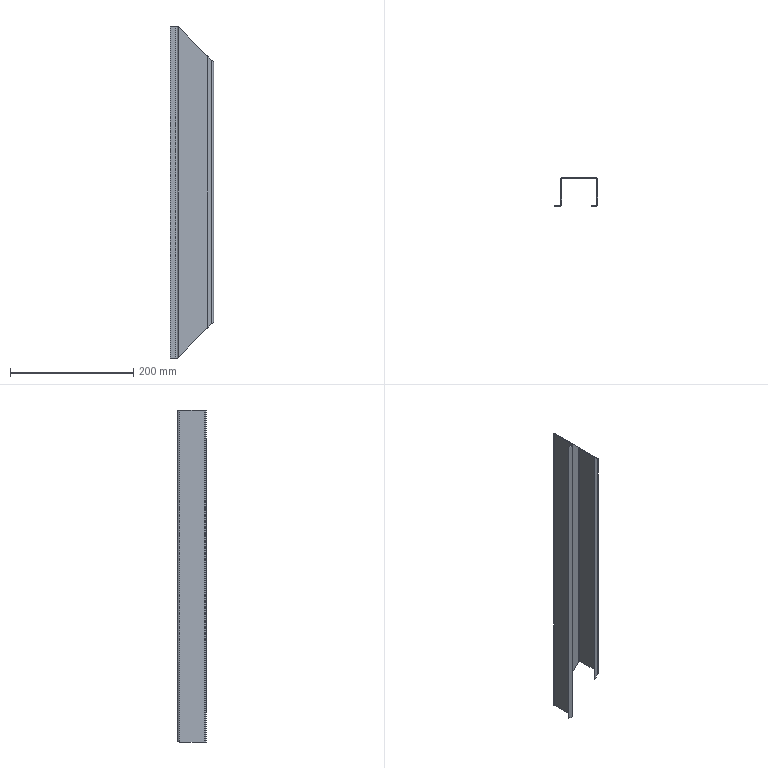Part | STEP file | 750078415 | 1 solid | 34 faces | box 70 x 46.5 x 539 mm | volume 119069 mm3 | plane 20 | cylinder 8 | spline 6 | commonest cylinder face diameters 3 x4 6 x4
STEP:
#1=CARTESIAN_POINT('',(-68.5,43.5,268.));
#2=VERTEX_POINT('',#1);
#3=CARTESIAN_POINT('',(-68.5,43.5,-268.));
#4=VERTEX_POINT('',#3);
#5=CARTESIAN_POINT('',(-68.5,43.5,269.5));
#6=DIRECTION('',(0.,0.,-1.));
#7=VECTOR('',#6,1000.);
#8=LINE('',#5,#7);
#9=EDGE_CURVE('',#2,#4,#8,.T.);
#10=ORIENTED_EDGE('',*,*,#9,.T.);
#11=CARTESIAN_POINT('',(-14.5,43.5,-214.));
#12=VERTEX_POINT('',#11);
#13=CARTESIAN_POINT('',(-68.5,43.5,-268.));
#14=DIRECTION('',(0.7071,0.,0.7071));
#15=VECTOR('',#14,1000.);
#16=LINE('',#13,#15);
#17=EDGE_CURVE('',#4,#12,#16,.T.);
#18=ORIENTED_EDGE('',*,*,#17,.T.);
#19=CARTESIAN_POINT('',(-14.5,43.5,214.));
#20=VERTEX_POINT('',#19);
#21=CARTESIAN_POINT('',(-14.5,43.5,269.5));
#22=DIRECTION('',(0.,0.,1.));
#23=VECTOR('',#22,1000.);
#24=LINE('',#21,#23);
#25=EDGE_CURVE('',#12,#20,#24,.T.);
#26=ORIENTED_EDGE('',*,*,#25,.T.);
#27=CARTESIAN_POINT('',(-14.5,43.5,214.));
#28=DIRECTION('',(-0.7071,0.,0.7071));
#29=VECTOR('',#28,1000.);
#30=LINE('',#27,#29);
#31=EDGE_CURVE('',#20,#2,#30,.T.);
#32=ORIENTED_EDGE('',*,*,#31,.T.);
#33=EDGE_LOOP('',(#10,#18,#26,#32));
#34=FACE_OUTER_BOUND('',#33,.T.);
#35=CARTESIAN_POINT('',(-11.5,43.5,269.5));
#36=DIRECTION('',(0.,-1.,0.));
#37=DIRECTION('',(1.,0.,0.));
#38=AXIS2_PLACEMENT_3D('',#35,#36,#37);
#39=PLANE('',#38);
#40=ADVANCED_FACE('',(#34),#39,.T.);
#41=CARTESIAN_POINT('',(-14.5,45.,-214.));
#42=VERTEX_POINT('',#41);
#43=CARTESIAN_POINT('',(-14.5,44.25,-214.));
#44=DIRECTION('',(0.,-1.,0.));
#45=VECTOR('',#44,1000.);
#46=LINE('',#43,#45);
#47=EDGE_CURVE('',#42,#12,#46,.T.);
#48=ORIENTED_EDGE('',*,*,#47,.T.);
#49=ORIENTED_EDGE('',*,*,#17,.F.);
#50=CARTESIAN_POINT('',(-68.5,45.,-268.));
#51=VERTEX_POINT('',#50);
#52=CARTESIAN_POINT('',(-68.5,44.25,-268.));
#53=DIRECTION('',(0.,1.,0.));
#54=VECTOR('',#53,1000.);
#55=LINE('',#52,#54);
#56=EDGE_CURVE('',#4,#51,#55,.T.);
#57=ORIENTED_EDGE('',*,*,#56,.T.);
#58=CARTESIAN_POINT('',(228.75,45.,29.25));
#59=DIRECTION('',(0.7071,0.,0.7071));
#60=VECTOR('',#59,1000.);
#61=LINE('',#58,#60);
#62=EDGE_CURVE('',#51,#42,#61,.T.);
#63=ORIENTED_EDGE('',*,*,#62,.T.);
#64=EDGE_LOOP('',(#48,#49,#57,#63));
#65=FACE_OUTER_BOUND('',#64,.T.);
#66=CARTESIAN_POINT('',(228.75,45.,29.25));
#67=DIRECTION('',(0.7071,0.,-0.7071));
#68=DIRECTION('',(-0.7071,0.,-0.7071));
#69=AXIS2_PLACEMENT_3D('',#66,#67,#68);
#70=PLANE('',#69);
#71=ADVANCED_FACE('',(#65),#70,.T.);
#72=CARTESIAN_POINT('',(-70.,42.,269.5));
#73=VERTEX_POINT('',#72);
#74=CARTESIAN_POINT('',(-70.,42.,269.5));
#75=CARTESIAN_POINT('',(-70.,42.75,269.5));
#76=CARTESIAN_POINT('',(-69.5,43.5,269.));
#77=CARTESIAN_POINT('',(-68.5,43.5,268.));
#78=(BOUNDED_CURVE()B_SPLINE_CURVE(3,(#74,#75,#76,#77),.UNSPECIFIED.,.F.,.F.)B_SPLINE_CURVE_WITH_KNOTS((4,4),(0.,0.002854),.UNSPECIFIED.)CURVE()GEOMETRIC_REPRESENTATION_ITEM()RATIONAL_B_SPLINE_CURVE((1.,0.6667,0.5,0.5))REPRESENTATION_ITEM(''));
#79=EDGE_CURVE('',#73,#2,#78,.T.);
#80=ORIENTED_EDGE('',*,*,#79,.F.);
#81=CARTESIAN_POINT('',(-70.,42.,-269.5));
#82=VERTEX_POINT('',#81);
#83=CARTESIAN_POINT('',(-70.,42.,269.5));
#84=DIRECTION('',(0.,0.,1.));
#85=VECTOR('',#84,1000.);
#86=LINE('',#83,#85);
#87=EDGE_CURVE('',#82,#73,#86,.T.);
#88=ORIENTED_EDGE('',*,*,#87,.F.);
#89=CARTESIAN_POINT('',(-68.5,43.5,-268.));
#90=CARTESIAN_POINT('',(-69.5,43.5,-269.));
#91=CARTESIAN_POINT('',(-70.,42.75,-269.5));
#92=CARTESIAN_POINT('',(-70.,42.,-269.5));
#93=(BOUNDED_CURVE()B_SPLINE_CURVE(3,(#89,#90,#91,#92),.UNSPECIFIED.,.F.,.F.)B_SPLINE_CURVE_WITH_KNOTS((4,4),(0.,0.002839),.UNSPECIFIED.)CURVE()GEOMETRIC_REPRESENTATION_ITEM()RATIONAL_B_SPLINE_CURVE((0.5,0.5,0.6667,1.))REPRESENTATION_ITEM(''));
#94=EDGE_CURVE('',#4,#82,#93,.T.);
#95=ORIENTED_EDGE('',*,*,#94,.F.);
#96=ORIENTED_EDGE('',*,*,#9,.F.);
#97=EDGE_LOOP('',(#80,#88,#95,#96));
#98=FACE_OUTER_BOUND('',#97,.T.);
#99=CARTESIAN_POINT('',(-68.5,42.,269.5));
#100=DIRECTION('',(0.,0.,-1.));
#101=DIRECTION('',(-1.,0.,0.));
#102=AXIS2_PLACEMENT_3D('',#99,#100,#101);
#103=CYLINDRICAL_SURFACE('',#102,1.5);
#104=ADVANCED_FACE('',(#98),#103,.F.);
#105=CARTESIAN_POINT('',(-68.5,45.,268.));
#106=VERTEX_POINT('',#105);
#107=CARTESIAN_POINT('',(-68.5,45.,268.));
#108=DIRECTION('',(0.,-1.,0.));
#109=VECTOR('',#108,1000.);
#110=LINE('',#107,#109);
#111=EDGE_CURVE('',#106,#2,#110,.T.);
#112=ORIENTED_EDGE('',*,*,#111,.T.);
#113=ORIENTED_EDGE('',*,*,#31,.F.);
#114=CARTESIAN_POINT('',(-14.5,45.,214.));
#115=VERTEX_POINT('',#114);
#116=CARTESIAN_POINT('',(-14.5,44.25,214.));
#117=DIRECTION('',(0.,1.,0.));
#118=VECTOR('',#117,1000.);
#119=LINE('',#116,#118);
#120=EDGE_CURVE('',#20,#115,#119,.T.);
#121=ORIENTED_EDGE('',*,*,#120,.T.);
#122=CARTESIAN_POINT('',(-40.75,45.,240.25));
#123=DIRECTION('',(-0.7071,0.,0.7071));
#124=VECTOR('',#123,1000.);
#125=LINE('',#122,#124);
#126=EDGE_CURVE('',#115,#106,#125,.T.);
#127=ORIENTED_EDGE('',*,*,#126,.T.);
#128=EDGE_LOOP('',(#112,#113,#121,#127));
#129=FACE_OUTER_BOUND('',#128,.T.);
#130=CARTESIAN_POINT('',(-40.75,45.,240.25));
#131=DIRECTION('',(0.7071,0.,0.7071));
#132=DIRECTION('',(0.7071,0.,-0.7071));
#133=AXIS2_PLACEMENT_3D('',#130,#131,#132);
#134=PLANE('',#133);
#135=ADVANCED_FACE('',(#129),#134,.T.);
#136=CARTESIAN_POINT('',(-13.,42.,211.));
#137=VERTEX_POINT('',#136);
#138=CARTESIAN_POINT('',(-14.5,43.5,214.));
#139=CARTESIAN_POINT('',(-13.5,43.5,212.));
#140=CARTESIAN_POINT('',(-13.,42.75,211.));
#141=CARTESIAN_POINT('',(-13.,42.,211.));
#142=(BOUNDED_CURVE()B_SPLINE_CURVE(3,(#138,#139,#140,#141),.UNSPECIFIED.,.F.,.F.)B_SPLINE_CURVE_WITH_KNOTS((4,4),(0.,0.003921),.UNSPECIFIED.)CURVE()GEOMETRIC_REPRESENTATION_ITEM()RATIONAL_B_SPLINE_CURVE((0.5,0.5,0.6667,1.))REPRESENTATION_ITEM(''));
#143=EDGE_CURVE('',#20,#137,#142,.T.);
#144=ORIENTED_EDGE('',*,*,#143,.F.);
#145=ORIENTED_EDGE('',*,*,#25,.F.);
#146=CARTESIAN_POINT('',(-13.,42.,-211.));
#147=VERTEX_POINT('',#146);
#148=CARTESIAN_POINT('',(-13.,42.,-211.));
#149=CARTESIAN_POINT('',(-13.,42.75,-211.));
#150=CARTESIAN_POINT('',(-13.5,43.5,-212.));
#151=CARTESIAN_POINT('',(-14.5,43.5,-214.));
#152=(BOUNDED_CURVE()B_SPLINE_CURVE(3,(#148,#149,#150,#151),.UNSPECIFIED.,.F.,.F.)B_SPLINE_CURVE_WITH_KNOTS((4,4),(0.,0.003968),.UNSPECIFIED.)CURVE()GEOMETRIC_REPRESENTATION_ITEM()RATIONAL_B_SPLINE_CURVE((1.,0.6667,0.5,0.5))REPRESENTATION_ITEM(''));
#153=EDGE_CURVE('',#147,#12,#152,.T.);
#154=ORIENTED_EDGE('',*,*,#153,.F.);
#155=CARTESIAN_POINT('',(-13.,42.,269.5));
#156=DIRECTION('',(0.,0.,-1.));
#157=VECTOR('',#156,1000.);
#158=LINE('',#155,#157);
#159=EDGE_CURVE('',#137,#147,#158,.T.);
#160=ORIENTED_EDGE('',*,*,#159,.F.);
#161=EDGE_LOOP('',(#144,#145,#154,#160));
#162=FACE_OUTER_BOUND('',#161,.T.);
#163=CARTESIAN_POINT('',(-14.5,42.,269.5));
#164=DIRECTION('',(0.,0.,-1.));
#165=DIRECTION('',(-1.,0.,0.));
#166=AXIS2_PLACEMENT_3D('',#163,#164,#165);
#167=CYLINDRICAL_SURFACE('',#166,1.5);
#168=ADVANCED_FACE('',(#162),#167,.F.);
#169=CARTESIAN_POINT('',(-14.5,45.,269.5));
#170=DIRECTION('',(0.,0.,1.));
#171=VECTOR('',#170,1000.);
#172=LINE('',#169,#171);
#173=EDGE_CURVE('',#42,#115,#172,.T.);
#174=ORIENTED_EDGE('',*,*,#173,.F.);
#175=ORIENTED_EDGE('',*,*,#62,.F.);
#176=CARTESIAN_POINT('',(-68.5,45.,269.5));
#177=DIRECTION('',(0.,0.,-1.));
#178=VECTOR('',#177,1000.);
#179=LINE('',#176,#178);
#180=EDGE_CURVE('',#106,#51,#179,.T.);
#181=ORIENTED_EDGE('',*,*,#180,.F.);
#182=ORIENTED_EDGE('',*,*,#126,.F.);
#183=EDGE_LOOP('',(#174,#175,#181,#182));
#184=FACE_OUTER_BOUND('',#183,.T.);
#185=CARTESIAN_POINT('',(-11.5,45.,269.5));
#186=DIRECTION('',(0.,-1.,0.));
#187=DIRECTION('',(1.,0.,0.));
#188=AXIS2_PLACEMENT_3D('',#185,#186,#187);
#189=PLANE('',#188);
#190=ADVANCED_FACE('',(#184),#189,.F.);
#191=ORIENTED_EDGE('',*,*,#79,.T.);
#192=ORIENTED_EDGE('',*,*,#111,.F.);
#193=CARTESIAN_POINT('',(-71.5,42.,269.5));
#194=VERTEX_POINT('',#193);
#195=CARTESIAN_POINT('',(-71.5,42.,269.5));
#196=CARTESIAN_POINT('',(-71.5,43.5,269.5));
#197=CARTESIAN_POINT('',(-70.5,45.,269.));
#198=CARTESIAN_POINT('',(-68.5,45.,268.));
#199=(BOUNDED_CURVE()B_SPLINE_CURVE(3,(#195,#196,#197,#198),.UNSPECIFIED.,.F.,.F.)B_SPLINE_CURVE_WITH_KNOTS((4,4),(0.,0.00499),.UNSPECIFIED.)CURVE()GEOMETRIC_REPRESENTATION_ITEM()RATIONAL_B_SPLINE_CURVE((1.,0.6667,0.5,0.5))REPRESENTATION_ITEM(''));
#200=EDGE_CURVE('',#194,#106,#199,.T.);
#201=ORIENTED_EDGE('',*,*,#200,.F.);
#202=CARTESIAN_POINT('',(-71.5,42.,269.5));
#203=DIRECTION('',(-1.,0.,0.));
#204=VECTOR('',#203,1000.);
#205=LINE('',#202,#204);
#206=EDGE_CURVE('',#73,#194,#205,.T.);
#207=ORIENTED_EDGE('',*,*,#206,.F.);
#208=EDGE_LOOP('',(#191,#192,#201,#207));
#209=FACE_OUTER_BOUND('',#208,.T.);
#210=CARTESIAN_POINT('',(-67.,42.,266.5));
#211=CARTESIAN_POINT('',(-66.5,42.,266.5));
#212=CARTESIAN_POINT('',(-66.,42.,266.5));
#213=CARTESIAN_POINT('',(-65.5,42.,266.5));
#214=CARTESIAN_POINT('',(-67.,45.,266.5));
#215=CARTESIAN_POINT('',(-66.5,46.,266.5));
#216=CARTESIAN_POINT('',(-66.,47.,266.5));
#217=CARTESIAN_POINT('',(-65.5,48.,266.5));
#218=CARTESIAN_POINT('',(-70.,45.,269.5));
#219=CARTESIAN_POINT('',(-70.5,46.,269.5));
#220=CARTESIAN_POINT('',(-71.,47.,269.5));
#221=CARTESIAN_POINT('',(-71.5,48.,269.5));
#222=CARTESIAN_POINT('',(-70.,42.,269.5));
#223=CARTESIAN_POINT('',(-70.5,42.,269.5));
#224=CARTESIAN_POINT('',(-71.,42.,269.5));
#225=CARTESIAN_POINT('',(-71.5,42.,269.5));
#226=CARTESIAN_POINT('',(-70.,39.,269.5));
#227=CARTESIAN_POINT('',(-70.5,38.,269.5));
#228=CARTESIAN_POINT('',(-71.,37.,269.5));
#229=CARTESIAN_POINT('',(-71.5,36.,269.5));
#230=CARTESIAN_POINT('',(-67.,39.,266.5));
#231=CARTESIAN_POINT('',(-66.5,38.,266.5));
#232=CARTESIAN_POINT('',(-66.,37.,266.5));
#233=CARTESIAN_POINT('',(-65.5,36.,266.5));
#234=CARTESIAN_POINT('',(-67.,42.,266.5));
#235=CARTESIAN_POINT('',(-66.5,42.,266.5));
#236=CARTESIAN_POINT('',(-66.,42.,266.5));
#237=CARTESIAN_POINT('',(-65.5,42.,266.5));
#238=(BOUNDED_SURFACE()B_SPLINE_SURFACE(3,3,((#210,#211,#212,#213),(#214,#215,#216,#217),(#218,#219,#220,#221),(#222,#223,#224,#225),(#226,#227,#228,#229),(#230,#231,#232,#233),(#234,#235,#236,#237)),.UNSPECIFIED.,.T.,.F.,.F.)B_SPLINE_SURFACE_WITH_KNOTS((4,3,4),(4,4),(0.,0.5,1.),(0.,1.),.UNSPECIFIED.)GEOMETRIC_REPRESENTATION_ITEM()RATIONAL_B_SPLINE_SURFACE(((1.,1.,1.,1.),(0.3333,0.3333,0.3333,0.3333),(0.3333,0.3333,0.3333,0.3333),(1.,1.,1.,1.),(0.3333,0.3333,0.3333,0.3333),(0.3333,0.3333,0.3333,0.3333),(1.,1.,1.,1.)))REPRESENTATION_ITEM('')SURFACE());
#239=ADVANCED_FACE('',(#209),#238,.F.);
#240=CARTESIAN_POINT('',(-70.,1.5,269.5));
#241=VERTEX_POINT('',#240);
#242=CARTESIAN_POINT('',(-70.,45.,269.5));
#243=DIRECTION('',(0.,-1.,0.));
#244=VECTOR('',#243,1000.);
#245=LINE('',#242,#244);
#246=EDGE_CURVE('',#73,#241,#245,.T.);
#247=ORIENTED_EDGE('',*,*,#246,.T.);
#248=CARTESIAN_POINT('',(-70.,1.5,-269.5));
#249=VERTEX_POINT('',#248);
#250=CARTESIAN_POINT('',(-70.,1.5,269.5));
#251=DIRECTION('',(0.,0.,-1.));
#252=VECTOR('',#251,1000.);
#253=LINE('',#250,#252);
#254=EDGE_CURVE('',#241,#249,#253,.T.);
#255=ORIENTED_EDGE('',*,*,#254,.T.);
#256=CARTESIAN_POINT('',(-70.,45.,-269.5));
#257=DIRECTION('',(0.,1.,0.));
#258=VECTOR('',#257,1000.);
#259=LINE('',#256,#258);
#260=EDGE_CURVE('',#249,#82,#259,.T.);
#261=ORIENTED_EDGE('',*,*,#260,.T.);
#262=ORIENTED_EDGE('',*,*,#87,.T.);
#263=EDGE_LOOP('',(#247,#255,#261,#262));
#264=FACE_OUTER_BOUND('',#263,.T.);
#265=CARTESIAN_POINT('',(-70.,45.,269.5));
#266=DIRECTION('',(1.,0.,0.));
#267=DIRECTION('',(0.,0.,-1.));
#268=AXIS2_PLACEMENT_3D('',#265,#266,#267);
#269=PLANE('',#268);
#270=ADVANCED_FACE('',(#264),#269,.T.);
#271=ORIENTED_EDGE('',*,*,#94,.T.);
#272=CARTESIAN_POINT('',(-71.5,42.,-269.5));
#273=VERTEX_POINT('',#272);
#274=CARTESIAN_POINT('',(-70.75,42.,-269.5));
#275=DIRECTION('',(1.,0.,0.));
#276=VECTOR('',#275,1000.);
#277=LINE('',#274,#276);
#278=EDGE_CURVE('',#273,#82,#277,.T.);
#279=ORIENTED_EDGE('',*,*,#278,.F.);
#280=CARTESIAN_POINT('',(-68.5,45.,-268.));
#281=CARTESIAN_POINT('',(-70.5,45.,-269.));
#282=CARTESIAN_POINT('',(-71.5,43.5,-269.5));
#283=CARTESIAN_POINT('',(-71.5,42.,-269.5));
#284=(BOUNDED_CURVE()B_SPLINE_CURVE(3,(#280,#281,#282,#283),.UNSPECIFIED.,.F.,.F.)B_SPLINE_CURVE_WITH_KNOTS((4,4),(0.,0.004967),.UNSPECIFIED.)CURVE()GEOMETRIC_REPRESENTATION_ITEM()RATIONAL_B_SPLINE_CURVE((0.5,0.5,0.6667,1.))REPRESENTATION_ITEM(''));
#285=EDGE_CURVE('',#51,#273,#284,.T.);
#286=ORIENTED_EDGE('',*,*,#285,.F.);
#287=ORIENTED_EDGE('',*,*,#56,.F.);
#288=EDGE_LOOP('',(#271,#279,#286,#287));
#289=FACE_OUTER_BOUND('',#288,.T.);
#290=CARTESIAN_POINT('',(-70.,42.,-269.5));
#291=CARTESIAN_POINT('',(-70.5,42.,-269.5));
#292=CARTESIAN_POINT('',(-71.,42.,-269.5));
#293=CARTESIAN_POINT('',(-71.5,42.,-269.5));
#294=CARTESIAN_POINT('',(-70.,45.,-269.5));
#295=CARTESIAN_POINT('',(-70.5,46.,-269.5));
#296=CARTESIAN_POINT('',(-71.,47.,-269.5));
#297=CARTESIAN_POINT('',(-71.5,48.,-269.5));
#298=CARTESIAN_POINT('',(-67.,45.,-266.5));
#299=CARTESIAN_POINT('',(-66.5,46.,-266.5));
#300=CARTESIAN_POINT('',(-66.,47.,-266.5));
#301=CARTESIAN_POINT('',(-65.5,48.,-266.5));
#302=CARTESIAN_POINT('',(-67.,42.,-266.5));
#303=CARTESIAN_POINT('',(-66.5,42.,-266.5));
#304=CARTESIAN_POINT('',(-66.,42.,-266.5));
#305=CARTESIAN_POINT('',(-65.5,42.,-266.5));
#306=CARTESIAN_POINT('',(-67.,39.,-266.5));
#307=CARTESIAN_POINT('',(-66.5,38.,-266.5));
#308=CARTESIAN_POINT('',(-66.,37.,-266.5));
#309=CARTESIAN_POINT('',(-65.5,36.,-266.5));
#310=CARTESIAN_POINT('',(-70.,39.,-269.5));
#311=CARTESIAN_POINT('',(-70.5,38.,-269.5));
#312=CARTESIAN_POINT('',(-71.,37.,-269.5));
#313=CARTESIAN_POINT('',(-71.5,36.,-269.5));
#314=CARTESIAN_POINT('',(-70.,42.,-269.5));
#315=CARTESIAN_POINT('',(-70.5,42.,-269.5));
#316=CARTESIAN_POINT('',(-71.,42.,-269.5));
#317=CARTESIAN_POINT('',(-71.5,42.,-269.5));
#318=(BOUNDED_SURFACE()B_SPLINE_SURFACE(3,3,((#290,#291,#292,#293),(#294,#295,#296,#297),(#298,#299,#300,#301),(#302,#303,#304,#305),(#306,#307,#308,#309),(#310,#311,#312,#313),(#314,#315,#316,#317)),.UNSPECIFIED.,.T.,.F.,.F.)B_SPLINE_SURFACE_WITH_KNOTS((4,3,4),(4,4),(0.,0.5,1.),(0.,1.),.UNSPECIFIED.)GEOMETRIC_REPRESENTATION_ITEM()RATIONAL_B_SPLINE_SURFACE(((1.,1.,1.,1.),(0.3333,0.3333,0.3333,0.3333),(0.3333,0.3333,0.3333,0.3333),(1.,1.,1.,1.),(0.3333,0.3333,0.3333,0.3333),(0.3333,0.3333,0.3333,0.3333),(1.,1.,1.,1.)))REPRESENTATION_ITEM('')SURFACE());
#319=ADVANCED_FACE('',(#289),#318,.F.);
#320=ORIENTED_EDGE('',*,*,#159,.T.);
#321=CARTESIAN_POINT('',(-13.,1.5,-211.));
#322=VERTEX_POINT('',#321);
#323=CARTESIAN_POINT('',(-13.,-1.5,-211.));
#324=DIRECTION('',(0.,-1.,0.));
#325=VECTOR('',#324,1000.);
#326=LINE('',#323,#325);
#327=EDGE_CURVE('',#147,#322,#326,.T.);
#328=ORIENTED_EDGE('',*,*,#327,.T.);
#329=CARTESIAN_POINT('',(-13.,1.5,211.));
#330=VERTEX_POINT('',#329);
#331=CARTESIAN_POINT('',(-13.,1.5,269.5));
#332=DIRECTION('',(0.,0.,1.));
#333=VECTOR('',#332,1000.);
#334=LINE('',#331,#333);
#335=EDGE_CURVE('',#322,#330,#334,.T.);
#336=ORIENTED_EDGE('',*,*,#335,.T.);
#337=CARTESIAN_POINT('',(-13.,-1.5,211.));
#338=DIRECTION('',(0.,1.,0.));
#339=VECTOR('',#338,1000.);
#340=LINE('',#337,#339);
#341=EDGE_CURVE('',#330,#137,#340,.T.);
#342=ORIENTED_EDGE('',*,*,#341,.T.);
#343=EDGE_LOOP('',(#320,#328,#336,#342));
#344=FACE_OUTER_BOUND('',#343,.T.);
#345=CARTESIAN_POINT('',(-13.,-1.5,269.5));
#346=DIRECTION('',(-1.,0.,0.));
#347=DIRECTION('',(0.,0.,1.));
#348=AXIS2_PLACEMENT_3D('',#345,#346,#347);
#349=PLANE('',#348);
#350=ADVANCED_FACE('',(#344),#349,.T.);
#351=CARTESIAN_POINT('',(-11.5,42.,211.));
#352=VERTEX_POINT('',#351);
#353=CARTESIAN_POINT('',(-14.5,45.,214.));
#354=CARTESIAN_POINT('',(-12.5,45.,212.));
#355=CARTESIAN_POINT('',(-11.5,43.5,211.));
#356=CARTESIAN_POINT('',(-11.5,42.,211.));
#357=(BOUNDED_CURVE()B_SPLINE_CURVE(3,(#353,#354,#355,#356),.UNSPECIFIED.,.F.,.F.)B_SPLINE_CURVE_WITH_KNOTS((4,4),(0.,0.005675),.UNSPECIFIED.)CURVE()GEOMETRIC_REPRESENTATION_ITEM()RATIONAL_B_SPLINE_CURVE((0.5,0.5,0.6667,1.))REPRESENTATION_ITEM(''));
#358=EDGE_CURVE('',#115,#352,#357,.T.);
#359=ORIENTED_EDGE('',*,*,#358,.F.);
#360=ORIENTED_EDGE('',*,*,#120,.F.);
#361=ORIENTED_EDGE('',*,*,#143,.T.);
#362=CARTESIAN_POINT('',(-12.25,42.,211.));
#363=DIRECTION('',(-1.,0.,0.));
#364=VECTOR('',#363,1000.);
#365=LINE('',#362,#364);
#366=EDGE_CURVE('',#352,#137,#365,.T.);
#367=ORIENTED_EDGE('',*,*,#366,.F.);
#368=EDGE_LOOP('',(#359,#360,#361,#367));
#369=FACE_OUTER_BOUND('',#368,.T.);
#370=CARTESIAN_POINT('',(-13.,42.,211.));
#371=CARTESIAN_POINT('',(-12.5,42.,211.));
#372=CARTESIAN_POINT('',(-12.,42.,211.));
#373=CARTESIAN_POINT('',(-11.5,42.,211.));
#374=CARTESIAN_POINT('',(-13.,45.,211.));
#375=CARTESIAN_POINT('',(-12.5,46.,211.));
#376=CARTESIAN_POINT('',(-12.,47.,211.));
#377=CARTESIAN_POINT('',(-11.5,48.,211.));
#378=CARTESIAN_POINT('',(-16.,45.,217.));
#379=CARTESIAN_POINT('',(-16.5,46.,217.));
#380=CARTESIAN_POINT('',(-17.,47.,217.));
#381=CARTESIAN_POINT('',(-17.5,48.,217.));
#382=CARTESIAN_POINT('',(-16.,42.,217.));
#383=CARTESIAN_POINT('',(-16.5,42.,217.));
#384=CARTESIAN_POINT('',(-17.,42.,217.));
#385=CARTESIAN_POINT('',(-17.5,42.,217.));
#386=CARTESIAN_POINT('',(-16.,39.,217.));
#387=CARTESIAN_POINT('',(-16.5,38.,217.));
#388=CARTESIAN_POINT('',(-17.,37.,217.));
#389=CARTESIAN_POINT('',(-17.5,36.,217.));
#390=CARTESIAN_POINT('',(-13.,39.,211.));
#391=CARTESIAN_POINT('',(-12.5,38.,211.));
#392=CARTESIAN_POINT('',(-12.,37.,211.));
#393=CARTESIAN_POINT('',(-11.5,36.,211.));
#394=CARTESIAN_POINT('',(-13.,42.,211.));
#395=CARTESIAN_POINT('',(-12.5,42.,211.));
#396=CARTESIAN_POINT('',(-12.,42.,211.));
#397=CARTESIAN_POINT('',(-11.5,42.,211.));
#398=(BOUNDED_SURFACE()B_SPLINE_SURFACE(3,3,((#370,#371,#372,#373),(#374,#375,#376,#377),(#378,#379,#380,#381),(#382,#383,#384,#385),(#386,#387,#388,#389),(#390,#391,#392,#393),(#394,#395,#396,#397)),.UNSPECIFIED.,.T.,.F.,.F.)B_SPLINE_SURFACE_WITH_KNOTS((4,3,4),(4,4),(0.,0.5,1.),(0.,1.),.UNSPECIFIED.)GEOMETRIC_REPRESENTATION_ITEM()RATIONAL_B_SPLINE_SURFACE(((1.,1.,1.,1.),(0.3333,0.3333,0.3333,0.3333),(0.3333,0.3333,0.3333,0.3333),(1.,1.,1.,1.),(0.3333,0.3333,0.3333,0.3333),(0.3333,0.3333,0.3333,0.3333),(1.,1.,1.,1.)))REPRESENTATION_ITEM('')SURFACE());
#399=ADVANCED_FACE('',(#369),#398,.F.);
#400=CARTESIAN_POINT('',(-11.5,42.,-211.));
#401=VERTEX_POINT('',#400);
#402=CARTESIAN_POINT('',(-11.5,42.,-211.));
#403=CARTESIAN_POINT('',(-11.5,43.5,-211.));
#404=CARTESIAN_POINT('',(-12.5,45.,-212.));
#405=CARTESIAN_POINT('',(-14.5,45.,-214.));
#406=(BOUNDED_CURVE()B_SPLINE_CURVE(3,(#402,#403,#404,#405),.UNSPECIFIED.,.F.,.F.)B_SPLINE_CURVE_WITH_KNOTS((4,4),(0.,0.005726),.UNSPECIFIED.)CURVE()GEOMETRIC_REPRESENTATION_ITEM()RATIONAL_B_SPLINE_CURVE((1.,0.6667,0.5,0.5))REPRESENTATION_ITEM(''));
#407=EDGE_CURVE('',#401,#42,#406,.T.);
#408=ORIENTED_EDGE('',*,*,#407,.F.);
#409=CARTESIAN_POINT('',(-12.25,42.,-211.));
#410=DIRECTION('',(1.,0.,0.));
#411=VECTOR('',#410,1000.);
#412=LINE('',#409,#411);
#413=EDGE_CURVE('',#147,#401,#412,.T.);
#414=ORIENTED_EDGE('',*,*,#413,.F.);
#415=ORIENTED_EDGE('',*,*,#153,.T.);
#416=ORIENTED_EDGE('',*,*,#47,.F.);
#417=EDGE_LOOP('',(#408,#414,#415,#416));
#418=FACE_OUTER_BOUND('',#417,.T.);
#419=CARTESIAN_POINT('',(-16.,42.,-217.));
#420=CARTESIAN_POINT('',(-16.5,42.,-217.));
#421=CARTESIAN_POINT('',(-17.,42.,-217.));
#422=CARTESIAN_POINT('',(-17.5,42.,-217.));
#423=CARTESIAN_POINT('',(-16.,45.,-217.));
#424=CARTESIAN_POINT('',(-16.5,46.,-217.));
#425=CARTESIAN_POINT('',(-17.,47.,-217.));
#426=CARTESIAN_POINT('',(-17.5,48.,-217.));
#427=CARTESIAN_POINT('',(-13.,45.,-211.));
#428=CARTESIAN_POINT('',(-12.5,46.,-211.));
#429=CARTESIAN_POINT('',(-12.,47.,-211.));
#430=CARTESIAN_POINT('',(-11.5,48.,-211.));
#431=CARTESIAN_POINT('',(-13.,42.,-211.));
#432=CARTESIAN_POINT('',(-12.5,42.,-211.));
#433=CARTESIAN_POINT('',(-12.,42.,-211.));
#434=CARTESIAN_POINT('',(-11.5,42.,-211.));
#435=CARTESIAN_POINT('',(-13.,39.,-211.));
#436=CARTESIAN_POINT('',(-12.5,38.,-211.));
#437=CARTESIAN_POINT('',(-12.,37.,-211.));
#438=CARTESIAN_POINT('',(-11.5,36.,-211.));
#439=CARTESIAN_POINT('',(-16.,39.,-217.));
#440=CARTESIAN_POINT('',(-16.5,38.,-217.));
#441=CARTESIAN_POINT('',(-17.,37.,-217.));
#442=CARTESIAN_POINT('',(-17.5,36.,-217.));
#443=CARTESIAN_POINT('',(-16.,42.,-217.));
#444=CARTESIAN_POINT('',(-16.5,42.,-217.));
#445=CARTESIAN_POINT('',(-17.,42.,-217.));
#446=CARTESIAN_POINT('',(-17.5,42.,-217.));
#447=(BOUNDED_SURFACE()B_SPLINE_SURFACE(3,3,((#419,#420,#421,#422),(#423,#424,#425,#426),(#427,#428,#429,#430),(#431,#432,#433,#434),(#435,#436,#437,#438),(#439,#440,#441,#442),(#443,#444,#445,#446)),.UNSPECIFIED.,.T.,.F.,.F.)B_SPLINE_SURFACE_WITH_KNOTS((4,3,4),(4,4),(0.,0.5,1.),(0.,1.),.UNSPECIFIED.)GEOMETRIC_REPRESENTATION_ITEM()RATIONAL_B_SPLINE_SURFACE(((1.,1.,1.,1.),(0.3333,0.3333,0.3333,0.3333),(0.3333,0.3333,0.3333,0.3333),(1.,1.,1.,1.),(0.3333,0.3333,0.3333,0.3333),(0.3333,0.3333,0.3333,0.3333),(1.,1.,1.,1.)))REPRESENTATION_ITEM('')SURFACE());
#448=ADVANCED_FACE('',(#418),#447,.F.);
#449=ORIENTED_EDGE('',*,*,#407,.T.);
#450=ORIENTED_EDGE('',*,*,#173,.T.);
#451=ORIENTED_EDGE('',*,*,#358,.T.);
#452=CARTESIAN_POINT('',(-11.5,42.,269.5));
#453=DIRECTION('',(0.,0.,-1.));
#454=VECTOR('',#453,1000.);
#455=LINE('',#452,#454);
#456=EDGE_CURVE('',#352,#401,#455,.T.);
#457=ORIENTED_EDGE('',*,*,#456,.T.);
#458=EDGE_LOOP('',(#449,#450,#451,#457));
#459=FACE_OUTER_BOUND('',#458,.T.);
#460=CARTESIAN_POINT('',(-14.5,42.,269.5));
#461=DIRECTION('',(0.,0.,-1.));
#462=DIRECTION('',(-1.,0.,0.));
#463=AXIS2_PLACEMENT_3D('',#460,#461,#462);
#464=CYLINDRICAL_SURFACE('',#463,3.);
#465=ADVANCED_FACE('',(#459),#464,.T.);
#466=ORIENTED_EDGE('',*,*,#285,.T.);
#467=CARTESIAN_POINT('',(-71.5,42.,269.5));
#468=DIRECTION('',(0.,0.,1.));
#469=VECTOR('',#468,1000.);
#470=LINE('',#467,#469);
#471=EDGE_CURVE('',#273,#194,#470,.T.);
#472=ORIENTED_EDGE('',*,*,#471,.T.);
#473=ORIENTED_EDGE('',*,*,#200,.T.);
#474=ORIENTED_EDGE('',*,*,#180,.T.);
#475=EDGE_LOOP('',(#466,#472,#473,#474));
#476=FACE_OUTER_BOUND('',#475,.T.);
#477=CARTESIAN_POINT('',(-68.5,42.,269.5));
#478=DIRECTION('',(0.,0.,-1.));
#479=DIRECTION('',(-1.,0.,0.));
#480=AXIS2_PLACEMENT_3D('',#477,#478,#479);
#481=CYLINDRICAL_SURFACE('',#480,3.);
#482=ADVANCED_FACE('',(#476),#481,.T.);
#483=CARTESIAN_POINT('',(-73.,-1.5,269.5));
#484=VERTEX_POINT('',#483);
#485=CARTESIAN_POINT('',(-73.,1.5,269.5));
#486=DIRECTION('',(0.,0.,-1.));
#487=DIRECTION('',(-1.,0.,0.));
#488=AXIS2_PLACEMENT_3D('',#485,#486,#487);
#489=CIRCLE('',#488,3.);
#490=EDGE_CURVE('',#241,#484,#489,.T.);
#491=ORIENTED_EDGE('',*,*,#490,.T.);
#492=CARTESIAN_POINT('',(-73.,-1.5,-269.5));
#493=VERTEX_POINT('',#492);
#494=CARTESIAN_POINT('',(-73.,-1.5,269.5));
#495=DIRECTION('',(0.,0.,-1.));
#496=VECTOR('',#495,1000.);
#497=LINE('',#494,#496);
#498=EDGE_CURVE('',#484,#493,#497,.T.);
#499=ORIENTED_EDGE('',*,*,#498,.T.);
#500=CARTESIAN_POINT('',(-73.,1.5,-269.5));
#501=DIRECTION('',(0.,0.,1.));
#502=DIRECTION('',(-1.,0.,0.));
#503=AXIS2_PLACEMENT_3D('',#500,#501,#502);
#504=CIRCLE('',#503,3.);
#505=EDGE_CURVE('',#493,#249,#504,.T.);
#506=ORIENTED_EDGE('',*,*,#505,.T.);
#507=ORIENTED_EDGE('',*,*,#254,.F.);
#508=EDGE_LOOP('',(#491,#499,#506,#507));
#509=FACE_OUTER_BOUND('',#508,.T.);
#510=CARTESIAN_POINT('',(-73.,1.5,269.5));
#511=DIRECTION('',(0.,0.,-1.));
#512=DIRECTION('',(-1.,0.,0.));
#513=AXIS2_PLACEMENT_3D('',#510,#511,#512);
#514=CYLINDRICAL_SURFACE('',#513,3.);
#515=ADVANCED_FACE('',(#509),#514,.T.);
#516=ORIENTED_EDGE('',*,*,#490,.F.);
#517=ORIENTED_EDGE('',*,*,#246,.F.);
#518=ORIENTED_EDGE('',*,*,#206,.T.);
#519=CARTESIAN_POINT('',(-71.5,1.5,269.5));
#520=VERTEX_POINT('',#519);
#521=CARTESIAN_POINT('',(-71.5,0.,269.5));
#522=DIRECTION('',(0.,-1.,0.));
#523=VECTOR('',#522,1000.);
#524=LINE('',#521,#523);
#525=EDGE_CURVE('',#194,#520,#524,.T.);
#526=ORIENTED_EDGE('',*,*,#525,.T.);
#527=CARTESIAN_POINT('',(-73.,0.,269.5));
#528=VERTEX_POINT('',#527);
#529=CARTESIAN_POINT('',(-73.,1.5,269.5));
#530=DIRECTION('',(0.,0.,-1.));
#531=DIRECTION('',(-1.,0.,0.));
#532=AXIS2_PLACEMENT_3D('',#529,#530,#531);
#533=CIRCLE('',#532,1.5);
#534=EDGE_CURVE('',#520,#528,#533,.T.);
#535=ORIENTED_EDGE('',*,*,#534,.T.);
#536=CARTESIAN_POINT('',(-81.5,0.,269.5));
#537=VERTEX_POINT('',#536);
#538=CARTESIAN_POINT('',(-71.5,0.,269.5));
#539=DIRECTION('',(-1.,0.,0.));
#540=VECTOR('',#539,1000.);
#541=LINE('',#538,#540);
#542=EDGE_CURVE('',#528,#537,#541,.T.);
#543=ORIENTED_EDGE('',*,*,#542,.T.);
#544=CARTESIAN_POINT('',(-81.5,-1.5,269.5));
#545=VERTEX_POINT('',#544);
#546=CARTESIAN_POINT('',(-81.5,0.,269.5));
#547=DIRECTION('',(0.,1.,0.));
#548=VECTOR('',#547,1000.);
#549=LINE('',#546,#548);
#550=EDGE_CURVE('',#545,#537,#549,.T.);
#551=ORIENTED_EDGE('',*,*,#550,.F.);
#552=CARTESIAN_POINT('',(-71.5,-1.5,269.5));
#553=DIRECTION('',(1.,0.,0.));
#554=VECTOR('',#553,1000.);
#555=LINE('',#552,#554);
#556=EDGE_CURVE('',#545,#484,#555,.T.);
#557=ORIENTED_EDGE('',*,*,#556,.T.);
#558=EDGE_LOOP('',(#516,#517,#518,#526,#535,#543,#551,#557));
#559=FACE_OUTER_BOUND('',#558,.T.);
#560=CARTESIAN_POINT('',(-71.5,0.,269.5));
#561=DIRECTION('',(0.,0.,1.));
#562=DIRECTION('',(1.,0.,0.));
#563=AXIS2_PLACEMENT_3D('',#560,#561,#562);
#564=PLANE('',#563);
#565=ADVANCED_FACE('',(#559),#564,.T.);
#566=ORIENTED_EDGE('',*,*,#278,.T.);
#567=ORIENTED_EDGE('',*,*,#260,.F.);
#568=ORIENTED_EDGE('',*,*,#505,.F.);
#569=CARTESIAN_POINT('',(-81.5,-1.5,-269.5));
#570=VERTEX_POINT('',#569);
#571=CARTESIAN_POINT('',(-21.5,-1.5,-269.5));
#572=DIRECTION('',(1.,0.,0.));
#573=VECTOR('',#572,1000.);
#574=LINE('',#571,#573);
#575=EDGE_CURVE('',#570,#493,#574,.T.);
#576=ORIENTED_EDGE('',*,*,#575,.F.);
#577=CARTESIAN_POINT('',(-81.5,0.,-269.5));
#578=VERTEX_POINT('',#577);
#579=CARTESIAN_POINT('',(-81.5,0.,-269.5));
#580=DIRECTION('',(0.,-1.,0.));
#581=VECTOR('',#580,1000.);
#582=LINE('',#579,#581);
#583=EDGE_CURVE('',#578,#570,#582,.T.);
#584=ORIENTED_EDGE('',*,*,#583,.F.);
#585=CARTESIAN_POINT('',(-73.,0.,-269.5));
#586=VERTEX_POINT('',#585);
#587=CARTESIAN_POINT('',(-21.5,0.,-269.5));
#588=DIRECTION('',(-1.,0.,0.));
#589=VECTOR('',#588,1000.);
#590=LINE('',#587,#589);
#591=EDGE_CURVE('',#586,#578,#590,.T.);
#592=ORIENTED_EDGE('',*,*,#591,.F.);
#593=CARTESIAN_POINT('',(-71.5,1.5,-269.5));
#594=VERTEX_POINT('',#593);
#595=CARTESIAN_POINT('',(-73.,1.5,-269.5));
#596=DIRECTION('',(0.,0.,-1.));
#597=DIRECTION('',(-1.,0.,0.));
#598=AXIS2_PLACEMENT_3D('',#595,#596,#597);
#599=CIRCLE('',#598,1.5);
#600=EDGE_CURVE('',#594,#586,#599,.T.);
#601=ORIENTED_EDGE('',*,*,#600,.F.);
#602=CARTESIAN_POINT('',(-71.5,-1.5,-269.5));
#603=DIRECTION('',(0.,-1.,0.));
#604=VECTOR('',#603,1000.);
#605=LINE('',#602,#604);
#606=EDGE_CURVE('',#273,#594,#605,.T.);
#607=ORIENTED_EDGE('',*,*,#606,.F.);
#608=EDGE_LOOP('',(#566,#567,#568,#576,#584,#592,#601,#607));
#609=FACE_OUTER_BOUND('',#608,.T.);
#610=CARTESIAN_POINT('',(-21.5,-1.5,-269.5));
#611=DIRECTION('',(0.,0.,1.));
#612=DIRECTION('',(1.,0.,0.));
#613=AXIS2_PLACEMENT_3D('',#610,#611,#612);
#614=PLANE('',#613);
#615=ADVANCED_FACE('',(#609),#614,.F.);
#616=CARTESIAN_POINT('',(-11.5,1.5,-211.));
#617=VERTEX_POINT('',#616);
#618=CARTESIAN_POINT('',(-12.25,1.5,-211.));
#619=DIRECTION('',(-1.,0.,0.));
#620=VECTOR('',#619,1000.);
#621=LINE('',#618,#620);
#622=EDGE_CURVE('',#617,#322,#621,.T.);
#623=ORIENTED_EDGE('',*,*,#622,.T.);
#624=ORIENTED_EDGE('',*,*,#327,.F.);
#625=ORIENTED_EDGE('',*,*,#413,.T.);
#626=CARTESIAN_POINT('',(-11.5,-1.5,-211.));
#627=DIRECTION('',(0.,-1.,0.));
#628=VECTOR('',#627,1000.);
#629=LINE('',#626,#628);
#630=EDGE_CURVE('',#401,#617,#629,.T.);
#631=ORIENTED_EDGE('',*,*,#630,.T.);
#632=EDGE_LOOP('',(#623,#624,#625,#631));
#633=FACE_OUTER_BOUND('',#632,.T.);
#634=CARTESIAN_POINT('',(-11.5,-1.5,-211.));
#635=DIRECTION('',(0.,0.,-1.));
#636=DIRECTION('',(-1.,0.,0.));
#637=AXIS2_PLACEMENT_3D('',#634,#635,#636);
#638=PLANE('',#637);
#639=ADVANCED_FACE('',(#633),#638,.T.);
#640=ORIENTED_EDGE('',*,*,#366,.T.);
#641=ORIENTED_EDGE('',*,*,#341,.F.);
#642=CARTESIAN_POINT('',(-11.5,1.5,211.));
#643=VERTEX_POINT('',#642);
#644=CARTESIAN_POINT('',(-12.25,1.5,211.));
#645=DIRECTION('',(1.,0.,0.));
#646=VECTOR('',#645,1000.);
#647=LINE('',#644,#646);
#648=EDGE_CURVE('',#330,#643,#647,.T.);
#649=ORIENTED_EDGE('',*,*,#648,.T.);
#650=CARTESIAN_POINT('',(-11.5,-1.5,211.));
#651=DIRECTION('',(0.,1.,0.));
#652=VECTOR('',#651,1000.);
#653=LINE('',#650,#652);
#654=EDGE_CURVE('',#643,#352,#653,.T.);
#655=ORIENTED_EDGE('',*,*,#654,.T.);
#656=EDGE_LOOP('',(#640,#641,#649,#655));
#657=FACE_OUTER_BOUND('',#656,.T.);
#658=CARTESIAN_POINT('',(-11.5,-1.5,211.));
#659=DIRECTION('',(0.,0.,1.));
#660=DIRECTION('',(1.,0.,0.));
#661=AXIS2_PLACEMENT_3D('',#658,#659,#660);
#662=PLANE('',#661);
#663=ADVANCED_FACE('',(#657),#662,.T.);
#664=CARTESIAN_POINT('',(-14.5,0.,214.));
#665=VERTEX_POINT('',#664);
#666=CARTESIAN_POINT('',(-13.,1.5,211.));
#667=CARTESIAN_POINT('',(-13.,0.75,211.));
#668=CARTESIAN_POINT('',(-13.5,0.,212.));
#669=CARTESIAN_POINT('',(-14.5,0.,214.));
#670=(BOUNDED_CURVE()B_SPLINE_CURVE(3,(#666,#667,#668,#669),.UNSPECIFIED.,.F.,.F.)B_SPLINE_CURVE_WITH_KNOTS((4,4),(0.,0.003968),.UNSPECIFIED.)CURVE()GEOMETRIC_REPRESENTATION_ITEM()RATIONAL_B_SPLINE_CURVE((1.,0.6667,0.5,0.5))REPRESENTATION_ITEM(''));
#671=EDGE_CURVE('',#330,#665,#670,.T.);
#672=ORIENTED_EDGE('',*,*,#671,.F.);
#673=ORIENTED_EDGE('',*,*,#335,.F.);
#674=CARTESIAN_POINT('',(-14.5,0.,-214.));
#675=VERTEX_POINT('',#674);
#676=CARTESIAN_POINT('',(-14.5,0.,-214.));
#677=CARTESIAN_POINT('',(-13.5,0.,-212.));
#678=CARTESIAN_POINT('',(-13.,0.75,-211.));
#679=CARTESIAN_POINT('',(-13.,1.5,-211.));
#680=(BOUNDED_CURVE()B_SPLINE_CURVE(3,(#676,#677,#678,#679),.UNSPECIFIED.,.F.,.F.)B_SPLINE_CURVE_WITH_KNOTS((4,4),(0.,0.003921),.UNSPECIFIED.)CURVE()GEOMETRIC_REPRESENTATION_ITEM()RATIONAL_B_SPLINE_CURVE((0.5,0.5,0.6667,1.))REPRESENTATION_ITEM(''));
#681=EDGE_CURVE('',#675,#322,#680,.T.);
#682=ORIENTED_EDGE('',*,*,#681,.F.);
#683=CARTESIAN_POINT('',(-14.5,0.,269.5));
#684=DIRECTION('',(0.,0.,-1.));
#685=VECTOR('',#684,1000.);
#686=LINE('',#683,#685);
#687=EDGE_CURVE('',#665,#675,#686,.T.);
#688=ORIENTED_EDGE('',*,*,#687,.F.);
#689=EDGE_LOOP('',(#672,#673,#682,#688));
#690=FACE_OUTER_BOUND('',#689,.T.);
#691=CARTESIAN_POINT('',(-14.5,1.5,269.5));
#692=DIRECTION('',(0.,0.,-1.));
#693=DIRECTION('',(-1.,0.,0.));
#694=AXIS2_PLACEMENT_3D('',#691,#692,#693);
#695=CYLINDRICAL_SURFACE('',#694,1.5);
#696=ADVANCED_FACE('',(#690),#695,.F.);
#697=CARTESIAN_POINT('',(-11.5,1.5,269.5));
#698=DIRECTION('',(0.,0.,1.));
#699=VECTOR('',#698,1000.);
#700=LINE('',#697,#699);
#701=EDGE_CURVE('',#617,#643,#700,.T.);
#702=ORIENTED_EDGE('',*,*,#701,.F.);
#703=ORIENTED_EDGE('',*,*,#630,.F.);
#704=ORIENTED_EDGE('',*,*,#456,.F.);
#705=ORIENTED_EDGE('',*,*,#654,.F.);
#706=EDGE_LOOP('',(#702,#703,#704,#705));
#707=FACE_OUTER_BOUND('',#706,.T.);
#708=CARTESIAN_POINT('',(-11.5,-1.5,269.5));
#709=DIRECTION('',(-1.,0.,0.));
#710=DIRECTION('',(0.,0.,1.));
#711=AXIS2_PLACEMENT_3D('',#708,#709,#710);
#712=PLANE('',#711);
#713=ADVANCED_FACE('',(#707),#712,.F.);
#714=CARTESIAN_POINT('',(-71.5,1.5,269.5));
#715=DIRECTION('',(0.,0.,-1.));
#716=VECTOR('',#715,1000.);
#717=LINE('',#714,#716);
#718=EDGE_CURVE('',#520,#594,#717,.T.);
#719=ORIENTED_EDGE('',*,*,#718,.F.);
#720=ORIENTED_EDGE('',*,*,#525,.F.);
#721=ORIENTED_EDGE('',*,*,#471,.F.);
#722=ORIENTED_EDGE('',*,*,#606,.T.);
#723=EDGE_LOOP('',(#719,#720,#721,#722));
#724=FACE_OUTER_BOUND('',#723,.T.);
#725=CARTESIAN_POINT('',(-71.5,45.,269.5));
#726=DIRECTION('',(1.,0.,0.));
#727=DIRECTION('',(0.,0.,-1.));
#728=AXIS2_PLACEMENT_3D('',#725,#726,#727);
#729=PLANE('',#728);
#730=ADVANCED_FACE('',(#724),#729,.F.);
#731=ORIENTED_EDGE('',*,*,#556,.F.);
#732=CARTESIAN_POINT('',(-81.5,-1.5,269.5));
#733=DIRECTION('',(0.,0.,-1.));
#734=VECTOR('',#733,1000.);
#735=LINE('',#732,#734);
#736=EDGE_CURVE('',#545,#570,#735,.T.);
#737=ORIENTED_EDGE('',*,*,#736,.T.);
#738=ORIENTED_EDGE('',*,*,#575,.T.);
#739=ORIENTED_EDGE('',*,*,#498,.F.);
#740=EDGE_LOOP('',(#731,#737,#738,#739));
#741=FACE_OUTER_BOUND('',#740,.T.);
#742=CARTESIAN_POINT('',(-71.5,-1.5,269.5));
#743=DIRECTION('',(0.,-1.,0.));
#744=DIRECTION('',(1.,0.,0.));
#745=AXIS2_PLACEMENT_3D('',#742,#743,#744);
#746=PLANE('',#745);
#747=ADVANCED_FACE('',(#741),#746,.T.);
#748=CARTESIAN_POINT('',(-81.5,0.,269.5));
#749=DIRECTION('',(0.,0.,-1.));
#750=VECTOR('',#749,1000.);
#751=LINE('',#748,#750);
#752=EDGE_CURVE('',#537,#578,#751,.T.);
#753=ORIENTED_EDGE('',*,*,#752,.F.);
#754=ORIENTED_EDGE('',*,*,#542,.F.);
#755=CARTESIAN_POINT('',(-73.,0.,269.5));
#756=DIRECTION('',(0.,0.,1.));
#757=VECTOR('',#756,1000.);
#758=LINE('',#755,#757);
#759=EDGE_CURVE('',#586,#528,#758,.T.);
#760=ORIENTED_EDGE('',*,*,#759,.F.);
#761=ORIENTED_EDGE('',*,*,#591,.T.);
#762=EDGE_LOOP('',(#753,#754,#760,#761));
#763=FACE_OUTER_BOUND('',#762,.T.);
#764=CARTESIAN_POINT('',(-71.5,0.,269.5));
#765=DIRECTION('',(0.,-1.,0.));
#766=DIRECTION('',(1.,0.,0.));
#767=AXIS2_PLACEMENT_3D('',#764,#765,#766);
#768=PLANE('',#767);
#769=ADVANCED_FACE('',(#763),#768,.F.);
#770=ORIENTED_EDGE('',*,*,#759,.T.);
#771=ORIENTED_EDGE('',*,*,#534,.F.);
#772=ORIENTED_EDGE('',*,*,#718,.T.);
#773=ORIENTED_EDGE('',*,*,#600,.T.);
#774=EDGE_LOOP('',(#770,#771,#772,#773));
#775=FACE_OUTER_BOUND('',#774,.T.);
#776=CARTESIAN_POINT('',(-73.,1.5,269.5));
#777=DIRECTION('',(0.,0.,-1.));
#778=DIRECTION('',(-1.,0.,0.));
#779=AXIS2_PLACEMENT_3D('',#776,#777,#778);
#780=CYLINDRICAL_SURFACE('',#779,1.5);
#781=ADVANCED_FACE('',(#775),#780,.F.);
#782=ORIENTED_EDGE('',*,*,#687,.T.);
#783=CARTESIAN_POINT('',(-21.5,0.,-221.));
#784=VERTEX_POINT('',#783);
#785=CARTESIAN_POINT('',(-14.5,0.,-214.));
#786=DIRECTION('',(-0.7071,0.,-0.7071));
#787=VECTOR('',#786,1000.);
#788=LINE('',#785,#787);
#789=EDGE_CURVE('',#675,#784,#788,.T.);
#790=ORIENTED_EDGE('',*,*,#789,.T.);
#791=CARTESIAN_POINT('',(-21.5,0.,221.));
#792=VERTEX_POINT('',#791);
#793=CARTESIAN_POINT('',(-21.5,0.,269.5));
#794=DIRECTION('',(0.,0.,1.));
#795=VECTOR('',#794,1000.);
#796=LINE('',#793,#795);
#797=EDGE_CURVE('',#784,#792,#796,.T.);
#798=ORIENTED_EDGE('',*,*,#797,.T.);
#799=CARTESIAN_POINT('',(-21.5,0.,221.));
#800=DIRECTION('',(0.7071,0.,-0.7071));
#801=VECTOR('',#800,1000.);
#802=LINE('',#799,#801);
#803=EDGE_CURVE('',#792,#665,#802,.T.);
#804=ORIENTED_EDGE('',*,*,#803,.T.);
#805=EDGE_LOOP('',(#782,#790,#798,#804));
#806=FACE_OUTER_BOUND('',#805,.T.);
#807=CARTESIAN_POINT('',(-21.5,0.,269.5));
#808=DIRECTION('',(0.,1.,0.));
#809=DIRECTION('',(-1.,0.,0.));
#810=AXIS2_PLACEMENT_3D('',#807,#808,#809);
#811=PLANE('',#810);
#812=ADVANCED_FACE('',(#806),#811,.T.);
#813=CARTESIAN_POINT('',(-14.5,-1.5,214.));
#814=VERTEX_POINT('',#813);
#815=CARTESIAN_POINT('',(-11.5,1.5,211.));
#816=CARTESIAN_POINT('',(-11.5,0.,211.));
#817=CARTESIAN_POINT('',(-12.5,-1.5,212.));
#818=CARTESIAN_POINT('',(-14.5,-1.5,214.));
#819=(BOUNDED_CURVE()B_SPLINE_CURVE(3,(#815,#816,#817,#818),.UNSPECIFIED.,.F.,.F.)B_SPLINE_CURVE_WITH_KNOTS((4,4),(0.,0.005784),.UNSPECIFIED.)CURVE()GEOMETRIC_REPRESENTATION_ITEM()RATIONAL_B_SPLINE_CURVE((1.,0.6667,0.5,0.5))REPRESENTATION_ITEM(''));
#820=EDGE_CURVE('',#643,#814,#819,.T.);
#821=ORIENTED_EDGE('',*,*,#820,.F.);
#822=ORIENTED_EDGE('',*,*,#648,.F.);
#823=ORIENTED_EDGE('',*,*,#671,.T.);
#824=CARTESIAN_POINT('',(-14.5,-0.75,214.));
#825=DIRECTION('',(0.,1.,0.));
#826=VECTOR('',#825,1000.);
#827=LINE('',#824,#826);
#828=EDGE_CURVE('',#814,#665,#827,.T.);
#829=ORIENTED_EDGE('',*,*,#828,.F.);
#830=EDGE_LOOP('',(#821,#822,#823,#829));
#831=FACE_OUTER_BOUND('',#830,.T.);
#832=CARTESIAN_POINT('',(-13.,1.5,211.));
#833=CARTESIAN_POINT('',(-12.5,1.5,211.));
#834=CARTESIAN_POINT('',(-12.,1.5,211.));
#835=CARTESIAN_POINT('',(-11.5,1.5,211.));
#836=CARTESIAN_POINT('',(-13.,4.5,211.));
#837=CARTESIAN_POINT('',(-12.5,5.5,211.));
#838=CARTESIAN_POINT('',(-12.,6.5,211.));
#839=CARTESIAN_POINT('',(-11.5,7.5,211.));
#840=CARTESIAN_POINT('',(-16.,4.5,217.));
#841=CARTESIAN_POINT('',(-16.5,5.5,217.));
#842=CARTESIAN_POINT('',(-17.,6.5,217.));
#843=CARTESIAN_POINT('',(-17.5,7.5,217.));
#844=CARTESIAN_POINT('',(-16.,1.5,217.));
#845=CARTESIAN_POINT('',(-16.5,1.5,217.));
#846=CARTESIAN_POINT('',(-17.,1.5,217.));
#847=CARTESIAN_POINT('',(-17.5,1.5,217.));
#848=CARTESIAN_POINT('',(-16.,-1.5,217.));
#849=CARTESIAN_POINT('',(-16.5,-2.5,217.));
#850=CARTESIAN_POINT('',(-17.,-3.5,217.));
#851=CARTESIAN_POINT('',(-17.5,-4.5,217.));
#852=CARTESIAN_POINT('',(-13.,-1.5,211.));
#853=CARTESIAN_POINT('',(-12.5,-2.5,211.));
#854=CARTESIAN_POINT('',(-12.,-3.5,211.));
#855=CARTESIAN_POINT('',(-11.5,-4.5,211.));
#856=CARTESIAN_POINT('',(-13.,1.5,211.));
#857=CARTESIAN_POINT('',(-12.5,1.5,211.));
#858=CARTESIAN_POINT('',(-12.,1.5,211.));
#859=CARTESIAN_POINT('',(-11.5,1.5,211.));
#860=(BOUNDED_SURFACE()B_SPLINE_SURFACE(3,3,((#832,#833,#834,#835),(#836,#837,#838,#839),(#840,#841,#842,#843),(#844,#845,#846,#847),(#848,#849,#850,#851),(#852,#853,#854,#855),(#856,#857,#858,#859)),.UNSPECIFIED.,.T.,.F.,.T.)B_SPLINE_SURFACE_WITH_KNOTS((4,3,4),(4,4),(0.,0.5,1.),(0.,1.),.UNSPECIFIED.)GEOMETRIC_REPRESENTATION_ITEM()RATIONAL_B_SPLINE_SURFACE(((1.,1.,1.,1.),(0.3333,0.3333,0.3333,0.3333),(0.3333,0.3333,0.3333,0.3333),(1.,1.,1.,1.),(0.3333,0.3333,0.3333,0.3333),(0.3333,0.3333,0.3333,0.3333),(1.,1.,1.,1.)))REPRESENTATION_ITEM('')SURFACE());
#861=ADVANCED_FACE('',(#831),#860,.F.);
#862=CARTESIAN_POINT('',(-14.5,-1.5,-214.));
#863=VERTEX_POINT('',#862);
#864=CARTESIAN_POINT('',(-14.5,-1.5,-214.));
#865=CARTESIAN_POINT('',(-12.5,-1.5,-212.));
#866=CARTESIAN_POINT('',(-11.5,0.,-211.));
#867=CARTESIAN_POINT('',(-11.5,1.5,-211.));
#868=(BOUNDED_CURVE()B_SPLINE_CURVE(3,(#864,#865,#866,#867),.UNSPECIFIED.,.F.,.F.)B_SPLINE_CURVE_WITH_KNOTS((4,4),(0.,0.005675),.UNSPECIFIED.)CURVE()GEOMETRIC_REPRESENTATION_ITEM()RATIONAL_B_SPLINE_CURVE((0.5,0.5,0.6667,1.))REPRESENTATION_ITEM(''));
#869=EDGE_CURVE('',#863,#617,#868,.T.);
#870=ORIENTED_EDGE('',*,*,#869,.F.);
#871=CARTESIAN_POINT('',(-14.5,-0.75,-214.));
#872=DIRECTION('',(0.,-1.,0.));
#873=VECTOR('',#872,1000.);
#874=LINE('',#871,#873);
#875=EDGE_CURVE('',#675,#863,#874,.T.);
#876=ORIENTED_EDGE('',*,*,#875,.F.);
#877=ORIENTED_EDGE('',*,*,#681,.T.);
#878=ORIENTED_EDGE('',*,*,#622,.F.);
#879=EDGE_LOOP('',(#870,#876,#877,#878));
#880=FACE_OUTER_BOUND('',#879,.T.);
#881=CARTESIAN_POINT('',(-16.,1.5,-217.));
#882=CARTESIAN_POINT('',(-16.5,1.5,-217.));
#883=CARTESIAN_POINT('',(-17.,1.5,-217.));
#884=CARTESIAN_POINT('',(-17.5,1.5,-217.));
#885=CARTESIAN_POINT('',(-16.,4.5,-217.));
#886=CARTESIAN_POINT('',(-16.5,5.5,-217.));
#887=CARTESIAN_POINT('',(-17.,6.5,-217.));
#888=CARTESIAN_POINT('',(-17.5,7.5,-217.));
#889=CARTESIAN_POINT('',(-13.,4.5,-211.));
#890=CARTESIAN_POINT('',(-12.5,5.5,-211.));
#891=CARTESIAN_POINT('',(-12.,6.5,-211.));
#892=CARTESIAN_POINT('',(-11.5,7.5,-211.));
#893=CARTESIAN_POINT('',(-13.,1.5,-211.));
#894=CARTESIAN_POINT('',(-12.5,1.5,-211.));
#895=CARTESIAN_POINT('',(-12.,1.5,-211.));
#896=CARTESIAN_POINT('',(-11.5,1.5,-211.));
#897=CARTESIAN_POINT('',(-13.,-1.5,-211.));
#898=CARTESIAN_POINT('',(-12.5,-2.5,-211.));
#899=CARTESIAN_POINT('',(-12.,-3.5,-211.));
#900=CARTESIAN_POINT('',(-11.5,-4.5,-211.));
#901=CARTESIAN_POINT('',(-16.,-1.5,-217.));
#902=CARTESIAN_POINT('',(-16.5,-2.5,-217.));
#903=CARTESIAN_POINT('',(-17.,-3.5,-217.));
#904=CARTESIAN_POINT('',(-17.5,-4.5,-217.));
#905=CARTESIAN_POINT('',(-16.,1.5,-217.));
#906=CARTESIAN_POINT('',(-16.5,1.5,-217.));
#907=CARTESIAN_POINT('',(-17.,1.5,-217.));
#908=CARTESIAN_POINT('',(-17.5,1.5,-217.));
#909=(BOUNDED_SURFACE()B_SPLINE_SURFACE(3,3,((#881,#882,#883,#884),(#885,#886,#887,#888),(#889,#890,#891,#892),(#893,#894,#895,#896),(#897,#898,#899,#900),(#901,#902,#903,#904),(#905,#906,#907,#908)),.UNSPECIFIED.,.T.,.F.,.F.)B_SPLINE_SURFACE_WITH_KNOTS((4,3,4),(4,4),(0.,0.5,1.),(0.,1.),.UNSPECIFIED.)GEOMETRIC_REPRESENTATION_ITEM()RATIONAL_B_SPLINE_SURFACE(((1.,1.,1.,1.),(0.3333,0.3333,0.3333,0.3333),(0.3333,0.3333,0.3333,0.3333),(1.,1.,1.,1.),(0.3333,0.3333,0.3333,0.3333),(0.3333,0.3333,0.3333,0.3333),(1.,1.,1.,1.)))REPRESENTATION_ITEM('')SURFACE());
#910=ADVANCED_FACE('',(#880),#909,.F.);
#911=ORIENTED_EDGE('',*,*,#869,.T.);
#912=ORIENTED_EDGE('',*,*,#701,.T.);
#913=ORIENTED_EDGE('',*,*,#820,.T.);
#914=CARTESIAN_POINT('',(-14.5,-1.5,269.5));
#915=DIRECTION('',(0.,0.,-1.));
#916=VECTOR('',#915,1000.);
#917=LINE('',#914,#916);
#918=EDGE_CURVE('',#814,#863,#917,.T.);
#919=ORIENTED_EDGE('',*,*,#918,.T.);
#920=EDGE_LOOP('',(#911,#912,#913,#919));
#921=FACE_OUTER_BOUND('',#920,.T.);
#922=CARTESIAN_POINT('',(-14.5,1.5,269.5));
#923=DIRECTION('',(0.,0.,-1.));
#924=DIRECTION('',(-1.,0.,0.));
#925=AXIS2_PLACEMENT_3D('',#922,#923,#924);
#926=CYLINDRICAL_SURFACE('',#925,3.);
#927=ADVANCED_FACE('',(#921),#926,.T.);
#928=ORIENTED_EDGE('',*,*,#583,.T.);
#929=ORIENTED_EDGE('',*,*,#736,.F.);
#930=ORIENTED_EDGE('',*,*,#550,.T.);
#931=ORIENTED_EDGE('',*,*,#752,.T.);
#932=EDGE_LOOP('',(#928,#929,#930,#931));
#933=FACE_OUTER_BOUND('',#932,.T.);
#934=CARTESIAN_POINT('',(-81.5,0.,269.5));
#935=DIRECTION('',(-1.,0.,0.));
#936=DIRECTION('',(0.,-1.,0.));
#937=AXIS2_PLACEMENT_3D('',#934,#935,#936);
#938=PLANE('',#937);
#939=ADVANCED_FACE('',(#933),#938,.T.);
#940=CARTESIAN_POINT('',(-21.5,-1.5,-221.));
#941=VERTEX_POINT('',#940);
#942=CARTESIAN_POINT('',(-21.5,-1.5,-221.));
#943=DIRECTION('',(0.,1.,0.));
#944=VECTOR('',#943,1000.);
#945=LINE('',#942,#944);
#946=EDGE_CURVE('',#941,#784,#945,.T.);
#947=ORIENTED_EDGE('',*,*,#946,.T.);
#948=ORIENTED_EDGE('',*,*,#789,.F.);
#949=ORIENTED_EDGE('',*,*,#875,.T.);
#950=CARTESIAN_POINT('',(223.75,-1.5,24.25));
#951=DIRECTION('',(-0.7071,0.,-0.7071));
#952=VECTOR('',#951,1000.);
#953=LINE('',#950,#952);
#954=EDGE_CURVE('',#863,#941,#953,.T.);
#955=ORIENTED_EDGE('',*,*,#954,.T.);
#956=EDGE_LOOP('',(#947,#948,#949,#955));
#957=FACE_OUTER_BOUND('',#956,.T.);
#958=CARTESIAN_POINT('',(223.75,-1.5,24.25));
#959=DIRECTION('',(0.7071,0.,-0.7071));
#960=DIRECTION('',(-0.7071,0.,-0.7071));
#961=AXIS2_PLACEMENT_3D('',#958,#959,#960);
#962=PLANE('',#961);
#963=ADVANCED_FACE('',(#957),#962,.T.);
#964=ORIENTED_EDGE('',*,*,#828,.T.);
#965=ORIENTED_EDGE('',*,*,#803,.F.);
#966=CARTESIAN_POINT('',(-21.5,-1.5,221.));
#967=VERTEX_POINT('',#966);
#968=CARTESIAN_POINT('',(-21.5,-1.5,221.));
#969=DIRECTION('',(0.,-1.,0.));
#970=VECTOR('',#969,1000.);
#971=LINE('',#968,#970);
#972=EDGE_CURVE('',#792,#967,#971,.T.);
#973=ORIENTED_EDGE('',*,*,#972,.T.);
#974=CARTESIAN_POINT('',(-45.75,-1.5,245.25));
#975=DIRECTION('',(0.7071,0.,-0.7071));
#976=VECTOR('',#975,1000.);
#977=LINE('',#974,#976);
#978=EDGE_CURVE('',#967,#814,#977,.T.);
#979=ORIENTED_EDGE('',*,*,#978,.T.);
#980=EDGE_LOOP('',(#964,#965,#973,#979));
#981=FACE_OUTER_BOUND('',#980,.T.);
#982=CARTESIAN_POINT('',(-45.75,-1.5,245.25));
#983=DIRECTION('',(0.7071,0.,0.7071));
#984=DIRECTION('',(0.7071,0.,-0.7071));
#985=AXIS2_PLACEMENT_3D('',#982,#983,#984);
#986=PLANE('',#985);
#987=ADVANCED_FACE('',(#981),#986,.T.);
#988=ORIENTED_EDGE('',*,*,#797,.F.);
#989=ORIENTED_EDGE('',*,*,#946,.F.);
#990=CARTESIAN_POINT('',(-21.5,-1.5,269.5));
#991=DIRECTION('',(0.,0.,-1.));
#992=VECTOR('',#991,1000.);
#993=LINE('',#990,#992);
#994=EDGE_CURVE('',#967,#941,#993,.T.);
#995=ORIENTED_EDGE('',*,*,#994,.F.);
#996=ORIENTED_EDGE('',*,*,#972,.F.);
#997=EDGE_LOOP('',(#988,#989,#995,#996));
#998=FACE_OUTER_BOUND('',#997,.T.);
#999=CARTESIAN_POINT('',(-21.5,-1.5,269.5));
#1000=DIRECTION('',(1.,0.,0.));
#1001=DIRECTION('',(0.,1.,0.));
#1002=AXIS2_PLACEMENT_3D('',#999,#1000,#1001);
#1003=PLANE('',#1002);
#1004=ADVANCED_FACE('',(#998),#1003,.F.);
#1005=ORIENTED_EDGE('',*,*,#994,.T.);
#1006=ORIENTED_EDGE('',*,*,#954,.F.);
#1007=ORIENTED_EDGE('',*,*,#918,.F.);
#1008=ORIENTED_EDGE('',*,*,#978,.F.);
#1009=EDGE_LOOP('',(#1005,#1006,#1007,#1008));
#1010=FACE_OUTER_BOUND('',#1009,.T.);
#1011=CARTESIAN_POINT('',(-21.5,-1.5,269.5));
#1012=DIRECTION('',(0.,1.,0.));
#1013=DIRECTION('',(-1.,0.,0.));
#1014=AXIS2_PLACEMENT_3D('',#1011,#1012,#1013);
#1015=PLANE('',#1014);
#1016=ADVANCED_FACE('',(#1010),#1015,.F.);
#1017=CLOSED_SHELL('',(#40,#71,#104,#135,#168,#190,#239,#270,#319,#350,#399,#448,#465,#482,#515,#565,#615,#639,#663,#696,#713,#730,#747,#769,#781,#812,#861,#910,#927,#939,#963,#987,#1004,#1016));
#1018=MANIFOLD_SOLID_BREP('',#1017);
#1019=CARTESIAN_POINT('',(0.,0.,0.));
#1020=DIRECTION('',(0.,0.,1.));
#1021=DIRECTION('',(1.,0.,0.));
#1022=AXIS2_PLACEMENT_3D('',#1019,#1020,#1021);
#1023=(LENGTH_UNIT()NAMED_UNIT(*)SI_UNIT(.MILLI.,.METRE.));
#1024=UNCERTAINTY_MEASURE_WITH_UNIT(LENGTH_MEASURE(0.00001),#1023,'','');
#1025=(NAMED_UNIT(*)PLANE_ANGLE_UNIT()SI_UNIT($,.RADIAN.));
#1026=(NAMED_UNIT(*)SI_UNIT($,.STERADIAN.)SOLID_ANGLE_UNIT());
#1027=(GEOMETRIC_REPRESENTATION_CONTEXT(3)GLOBAL_UNCERTAINTY_ASSIGNED_CONTEXT((#1024))GLOBAL_UNIT_ASSIGNED_CONTEXT((#1023,#1025,#1026))REPRESENTATION_CONTEXT('',''));
#1028=ADVANCED_BREP_SHAPE_REPRESENTATION('',(#1018,#1022),#1027);